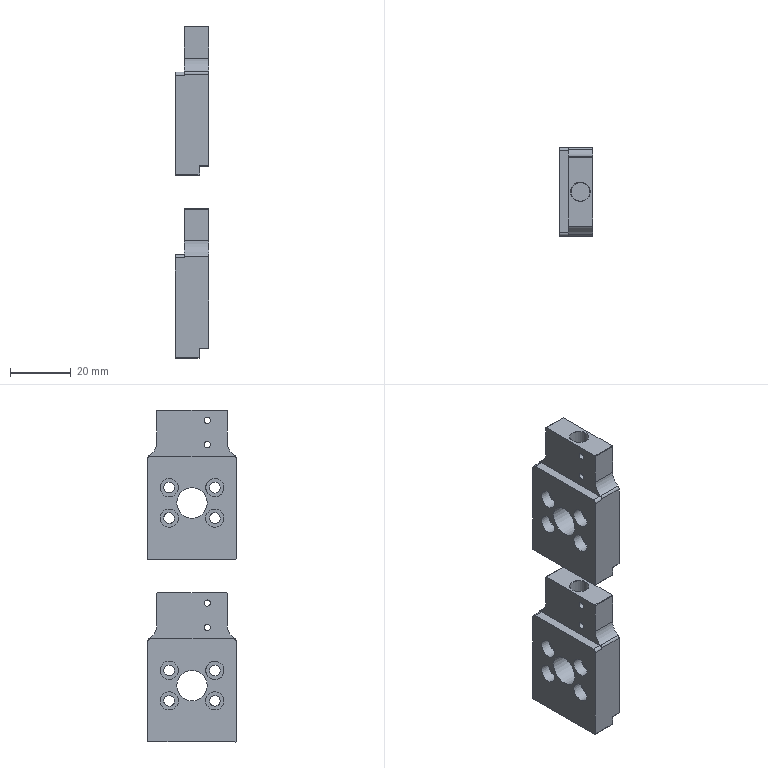CAM job | NX | 3+2 milling, drilling | part box 11 x 29 x 109 mm | stock box 15 x 30 x 114 mm
Tools:
number,name,description,diameter,corner_radius,flute_length,length,flutes
4,D4,平底铣刀-粗,4.0,0.0,25.0,75.0,2
6,D6,平底铣刀-粗,6.0,0.0,25.0,75.0,2
9,D10,平底铣刀-粗,10.0,0.0,35.0,75.0,2
7,D6-J,平底铣刀-精,6.0,0.0,25.0,75.0,2
10,D10-J,平底铣刀-精,10.0,0.0,35.0,75.0,2
1,D80R0.8飞刀,圆鼻刀-粗,80.0,0.8,50.0,75.0,2
1,D80R0.8飞刀-J,圆鼻刀-精,80.0,0.8,50.0,75.0,2
2,D6倒角刀,倒角刀,6.0,0.0,3.0,25.0,2
23,M2.5X0.45,丝锥,2.05,0.0,35.0,50.0,2
17,ZT2.1,钻头,2.1,0.0,35.0,50.0,2
18,ZT3.5,钻头,3.5,0.0,35.0,50.0,2
19,ZT9.8,Drilling Tool,9.8,0.0,35.0,50.0,2
Operations:
program,operation,operation_type,tool,method,geometry_group,spindle_rpm,surface_speed,feed_per_tooth,feed_cut,feed_plunge,cut_length_mm,path_length_mm,cut_time_min,machine_time_min
B,FLOOR_FACEMILL_1PASS_ROUGH_COPY,VolumeBased25DMillingOperation,D80R0.8飞刀,LAYER_ROUGH-DEPTHK-STEPG,W-B,2800.0,703.696,0.5357,3000.0,100.0,1520.358,2935.438,0.5068,0.6483
B,FLOOR_FACEMILL_1PASS_FINISH_COPY,VolumeBased25DMillingOperation,D80R0.8飞刀-J,SIDEEDGE_FINISH-DEPTHK-STEPG,W-B,4000.0,1005.28,0.125,1000.0,100.0,216.998,252.998,0.217,0.2206
B,FLOOR_LAYER_ROUGH-MED_COPY,VolumeBased25DMillingOperation,D6,LAYER_ROUGH-DEPTHK-STEPG,W-B,8000.0,150.796,0.1875,3000.0,100.0,4931.572,5070.347,1.644,1.658
B,FLOOR_FINISH_BOTTOMFACE-MED_COPY,VolumeBased25DMillingOperation,D6-J,FINISH_STEPDEPTH_OFF,W-B,8000.0,150.792,0.0625,1000.0,100.0,491.161,623.096,0.4912,0.5044
B,DRILL_CHAMFER_3,Operation,D6倒角刀,METHOD,W-B,8000.0,150.796,0.0625,1000.0,0.0,8.7,120.475,0.0087,0.0199
B,MILL_CHAMFER_3,PlanarMilling,D6倒角刀,METHOD,W-B,8000.0,150.796,0.075,1200.0,100.0,74.885,229.184,0.0624,0.0778
B,PLANAR_DEBURR_6X45L_COPY,SurfaceContour,D6倒角刀,WALLCLIMB_CHAMFER-DEPTH0-STEPG,W-B,6500.0,122.519,0.1154,1500.0,100.0,623.618,1113.358,0.4157,0.4647
B,FLOOR_FINISH_SIDE-MED-SELBOTTOM_COPY,VolumeBased25DMillingOperation,D6-J,SIDEEDGE_FINISH-DEPTHK-STEPG,W-B,8000.0,150.792,0.0625,1000.0,100.0,222.733,355.638,0.2227,0.236
A,TOP_FACE,FaceMilling,D80R0.8飞刀,SIDEEDGE_FINISH-DEPTHK-STEPG,W-A,4000.0,1005.31,0.125,1000.0,100.0,203.0,239.0,0.203,0.2066
A,CONTOUR_ROUGH_2,VolumeBased25DMillingOperation,D10,METHOD,W-A,8000.0,251.327,0.3125,5000.0,80.0,5886.111,6046.211,1.177,1.193
A,FLOOR_ROUGH_1,VolumeBased25DMillingOperation,D10,METHOD,W-A,6000.0,113.0,0.2083,3500.0,100.0,1497.353,1740.885,0.4278,0.4522
A,SPOT-DEPTH0.8,Operation,D6倒角刀,NONE,W-A,8000.0,150.796,0.0312,500.0,90.0,25.2,258.751,0.0504,0.0738
A,SPOT-DEPTH0.8_2,Operation,D6倒角刀,NONE,W-A,8000.0,150.796,0.0312,500.0,90.0,7.2,131.534,0.0144,0.0268
A,THROUGH_M2.5_TAPDRILL,Operation,ZT2.1,NONE,W-A,3000.0,19.792,0.0333,200.0,90.0,48.524,214.181,0.2426,0.2592
A,COUNTERBORE_DRILL_SEG0,Operation,ZT3.5,NONE,W-A,2800.0,30.788,0.0179,100.0,90.0,96.412,360.1,0.9641,0.9905
A,THROUGH_FINISHBORE10.0_PREDRILL,Operation,ZT9.8,NONE,W-A,1000.0,31.102,0.15,300.0,90.0,29.658,160.324,0.0989,0.1119
A,HOLE_ROUGH_D6_1,CylinderMilling,D6,NONE,W-A,8000.0,150.796,0.0625,1000.0,100.0,475.755,631.755,0.4758,0.4914
A,HOLE_ROUGH_D4_1,CylinderMilling,D4,NONE,W-A,8000.0,100.531,0.075,1200.0,100.0,671.892,1135.892,0.5599,0.6063
A,HOLE_FINISH_D4_1,CylinderMilling,D4,FINISH_STEPDEPTH_OFF,W-A,8000.0,100.531,0.0312,500.0,100.0,125.952,589.952,0.2519,0.2983
A,FLOOR_FINISH_1,VolumeBased25DMillingOperation,D6-J,METHOD,W-A,6000.0,113.0,0.2083,1200.0,100.0,275.681,438.156,0.2297,0.246
A,HOLE_FINISH_D6-J_1,CylinderMilling,D6-J,FINISH_STEPDEPTH_OFF,W-A,8000.0,150.796,0.0312,500.0,100.0,86.672,242.672,0.1733,0.1889
A,FLOOR_SIDE_FINISH_3,VolumeBased25DMillingOperation,D6-J,METHOD,W-A,6000.0,113.0,0.2083,1200.0,100.0,98.616,259.192,0.0822,0.0982
A,SELECTED_BODY_ONLY,SurfaceContour,D6倒角刀,METHOD,W-A,8000.0,150.796,0.1875,3000.0,100.0,412.399,709.097,0.1375,0.1671
A,DRILL_CHAMFER_1,Operation,D6倒角刀,METHOD,W-A,8000.0,150.796,0.0312,500.0,0.0,17.4,158.975,0.0348,0.049
A,MILL_CHAMFER_1,PlanarMilling,D6倒角刀,NONE,W-A,8000.0,150.796,0.0312,500.0,100.0,221.477,634.183,0.443,0.4842
A,MILL_CHAMFER_2,PlanarMilling,D6倒角刀,METHOD,W-A,8000.0,150.796,0.0312,500.0,100.0,74.885,217.184,0.1498,0.164
A,DRILL_CHAMFER_2,Operation,D6倒角刀,METHOD,W-A,8000.0,150.796,0.0312,500.0,0.0,18.0,160.174,0.036,0.0502
A,THROUGH_TAP_M2.5,Operation,M2.5X0.45,METHOD,W-A,1000.0,6.44,0.0002,0.45,90.0,42.0,201.134,93.333,93.349
A,CONTOUR_SEMIFINISH_2,VolumeBased25DMillingOperation,D10-J,METHOD,W-A,8000.0,251.327,0.0625,1000.0,100.0,376.477,545.559,0.3765,0.3934